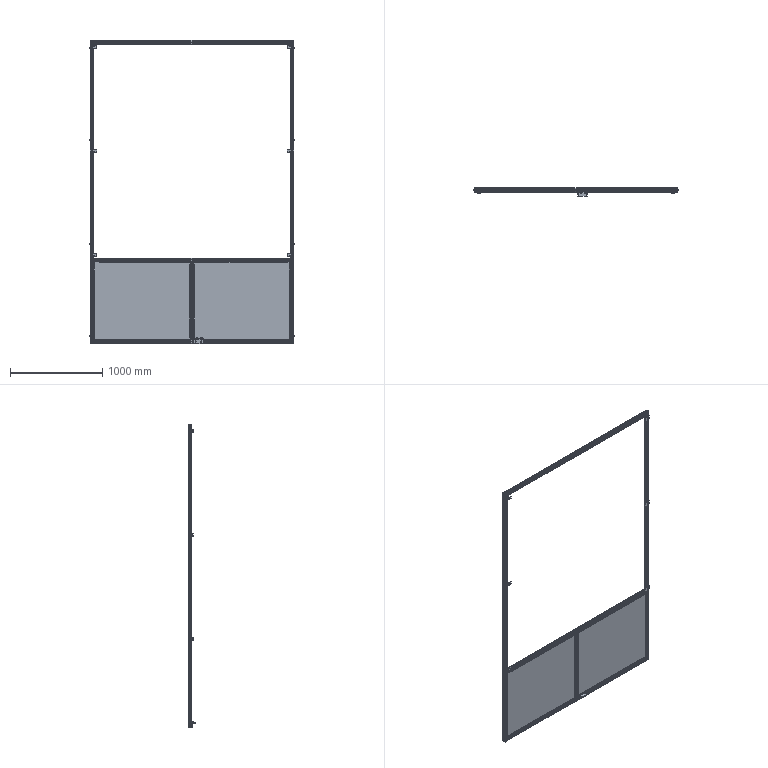Part | SolidWorks | features ReferencePattern 36, LocalLPattern 3, DerivedHolePattern 1, MirrorCompFeat 1 | 89 solids | 3666 faces | volume 17892849 mm3 | plane 2308 | cylinder 1064 | cone 278 | spline 16 | commonest cylinder face diameters 6.8 x178 5 x160 8 x76 2 x68 19 x48 1 x36